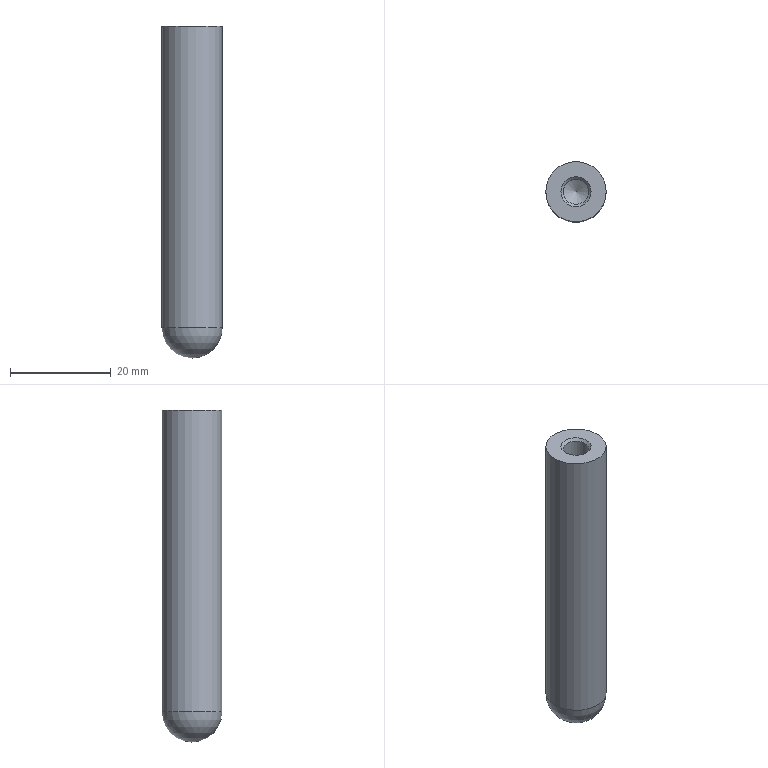Part | STEP file | gslz 2016.10.28-6_id74_x_t | 1 solid | 6 faces | box 12 x 12 x 66 mm | volume 6932 mm3 | cylinder 2 | cone 2 | plane 1 | sphere 1 | commonest cylinder face diameters 5 x1 12 x1
STEP:
#1=CARTESIAN_POINT('',(-242.,250.,-20.));
#2=VERTEX_POINT('',#1);
#3=CARTESIAN_POINT('',(-245.,250.,-20.));
#4=DIRECTION('',(0.,0.,-1.));
#5=DIRECTION('',(1.,0.,0.));
#6=AXIS2_PLACEMENT_3D('',#3,#4,#5);
#7=CIRCLE('',#6,3.);
#8=EDGE_CURVE('',#2,#2,#7,.T.);
#9=ORIENTED_EDGE('',*,*,#8,.T.);
#10=EDGE_LOOP('',(#9));
#11=FACE_BOUND('',#10,.T.);
#12=CARTESIAN_POINT('',(-251.,250.,-20.));
#13=VERTEX_POINT('',#12);
#14=CARTESIAN_POINT('',(-245.,250.,-20.));
#15=DIRECTION('',(0.,0.,-1.));
#16=DIRECTION('',(-1.,0.,0.));
#17=AXIS2_PLACEMENT_3D('',#14,#15,#16);
#18=CIRCLE('',#17,6.);
#19=EDGE_CURVE('',#13,#13,#18,.T.);
#20=ORIENTED_EDGE('',*,*,#19,.F.);
#21=EDGE_LOOP('',(#20));
#22=FACE_BOUND('',#21,.T.);
#23=CARTESIAN_POINT('',(-245.,250.,-20.));
#24=DIRECTION('',(0.,0.,1.));
#25=DIRECTION('',(-1.,0.,0.));
#26=AXIS2_PLACEMENT_3D('',#23,#24,#25);
#27=PLANE('',#26);
#28=ADVANCED_FACE('',(#11,#22),#27,.T.);
#29=CARTESIAN_POINT('',(-251.,250.,-80.));
#30=VERTEX_POINT('',#29);
#31=CARTESIAN_POINT('',(-245.,250.,-80.));
#32=DIRECTION('',(0.,0.,-1.));
#33=DIRECTION('',(-1.,0.,0.));
#34=AXIS2_PLACEMENT_3D('',#31,#32,#33);
#35=CIRCLE('',#34,6.);
#36=EDGE_CURVE('',#30,#30,#35,.T.);
#37=ORIENTED_EDGE('',*,*,#36,.F.);
#38=EDGE_LOOP('',(#37));
#39=FACE_BOUND('',#38,.T.);
#40=ORIENTED_EDGE('',*,*,#19,.T.);
#41=EDGE_LOOP('',(#40));
#42=FACE_BOUND('',#41,.T.);
#43=CARTESIAN_POINT('',(-245.,250.,-35.));
#44=DIRECTION('',(0.,0.,-1.));
#45=DIRECTION('',(-1.,0.,0.));
#46=AXIS2_PLACEMENT_3D('',#43,#44,#45);
#47=CYLINDRICAL_SURFACE('',#46,6.);
#48=ADVANCED_FACE('',(#39,#42),#47,.T.);
#49=ORIENTED_EDGE('',*,*,#36,.T.);
#50=EDGE_LOOP('',(#49));
#51=FACE_OUTER_BOUND('',#50,.T.);
#52=CARTESIAN_POINT('',(-245.,250.,-80.));
#53=DIRECTION('',(0.,0.,1.));
#54=DIRECTION('',(1.,0.,0.));
#55=AXIS2_PLACEMENT_3D('',#52,#53,#54);
#56=SPHERICAL_SURFACE('',#55,6.);
#57=ADVANCED_FACE('',(#51),#56,.T.);
#58=CARTESIAN_POINT('',(-247.5,250.,-35.));
#59=VERTEX_POINT('',#58);
#60=CARTESIAN_POINT('',(-245.,250.,-35.));
#61=DIRECTION('',(0.,0.,1.));
#62=DIRECTION('',(-1.,0.,0.));
#63=AXIS2_PLACEMENT_3D('',#60,#61,#62);
#64=CIRCLE('',#63,2.5);
#65=EDGE_CURVE('',#59,#59,#64,.T.);
#66=ORIENTED_EDGE('',*,*,#65,.T.);
#67=EDGE_LOOP('',(#66));
#68=FACE_BOUND('',#67,.T.);
#69=CARTESIAN_POINT('',(-245.,250.,-36.502));
#70=VERTEX_POINT('',#69);
#71=VERTEX_LOOP('',#70);
#72=FACE_BOUND('',#71,.T.);
#73=CARTESIAN_POINT('',(-245.,250.,-35.));
#74=DIRECTION('',(0.,0.,1.));
#75=DIRECTION('',(1.,0.,0.));
#76=AXIS2_PLACEMENT_3D('',#73,#74,#75);
#77=CONICAL_SURFACE('',#76,2.5,59.);
#78=ADVANCED_FACE('',(#68,#72),#77,.F.);
#79=CARTESIAN_POINT('',(-242.5,250.,-20.5));
#80=VERTEX_POINT('',#79);
#81=CARTESIAN_POINT('',(-245.,250.,-20.5));
#82=DIRECTION('',(0.,0.,1.));
#83=DIRECTION('',(1.,0.,0.));
#84=AXIS2_PLACEMENT_3D('',#81,#82,#83);
#85=CIRCLE('',#84,2.5);
#86=EDGE_CURVE('',#80,#80,#85,.T.);
#87=ORIENTED_EDGE('',*,*,#86,.T.);
#88=EDGE_LOOP('',(#87));
#89=FACE_BOUND('',#88,.T.);
#90=ORIENTED_EDGE('',*,*,#65,.F.);
#91=EDGE_LOOP('',(#90));
#92=FACE_BOUND('',#91,.T.);
#93=CARTESIAN_POINT('',(-245.,250.,-20.));
#94=DIRECTION('',(0.,0.,-1.));
#95=DIRECTION('',(-1.,0.,0.));
#96=AXIS2_PLACEMENT_3D('',#93,#94,#95);
#97=CYLINDRICAL_SURFACE('',#96,2.5);
#98=ADVANCED_FACE('',(#89,#92),#97,.F.);
#99=ORIENTED_EDGE('',*,*,#86,.F.);
#100=EDGE_LOOP('',(#99));
#101=FACE_BOUND('',#100,.T.);
#102=ORIENTED_EDGE('',*,*,#8,.F.);
#103=EDGE_LOOP('',(#102));
#104=FACE_BOUND('',#103,.T.);
#105=CARTESIAN_POINT('',(-245.,250.,-20.));
#106=DIRECTION('',(0.,0.,1.));
#107=DIRECTION('',(1.,0.,0.));
#108=AXIS2_PLACEMENT_3D('',#105,#106,#107);
#109=CONICAL_SURFACE('',#108,3.,45.);
#110=ADVANCED_FACE('',(#101,#104),#109,.F.);
#111=CLOSED_SHELL('',(#28,#48,#57,#78,#98,#110));
#112=MANIFOLD_SOLID_BREP('',#111);
#113=(LENGTH_UNIT()NAMED_UNIT(*)SI_UNIT(.MILLI.,.METRE.));
#114=UNCERTAINTY_MEASURE_WITH_UNIT(LENGTH_MEASURE(0.00002),#113,'','');
#115=(NAMED_UNIT(*)PLANE_ANGLE_UNIT()SI_UNIT($,.RADIAN.));
#116=PLANE_ANGLE_MEASURE_WITH_UNIT(PLANE_ANGLE_MEASURE(0.01745),#115);
#117=DIMENSIONAL_EXPONENTS(0.,0.,0.,0.,0.,0.,0.);
#118=(CONVERSION_BASED_UNIT('DEGREE',#116)NAMED_UNIT(#117)PLANE_ANGLE_UNIT());
#119=(NAMED_UNIT(*)SI_UNIT($,.STERADIAN.)SOLID_ANGLE_UNIT());
#120=(GEOMETRIC_REPRESENTATION_CONTEXT(3)GLOBAL_UNCERTAINTY_ASSIGNED_CONTEXT((#114))GLOBAL_UNIT_ASSIGNED_CONTEXT((#113,#118,#119))REPRESENTATION_CONTEXT('',''));
#121=ADVANCED_BREP_SHAPE_REPRESENTATION('',(#112),#120);